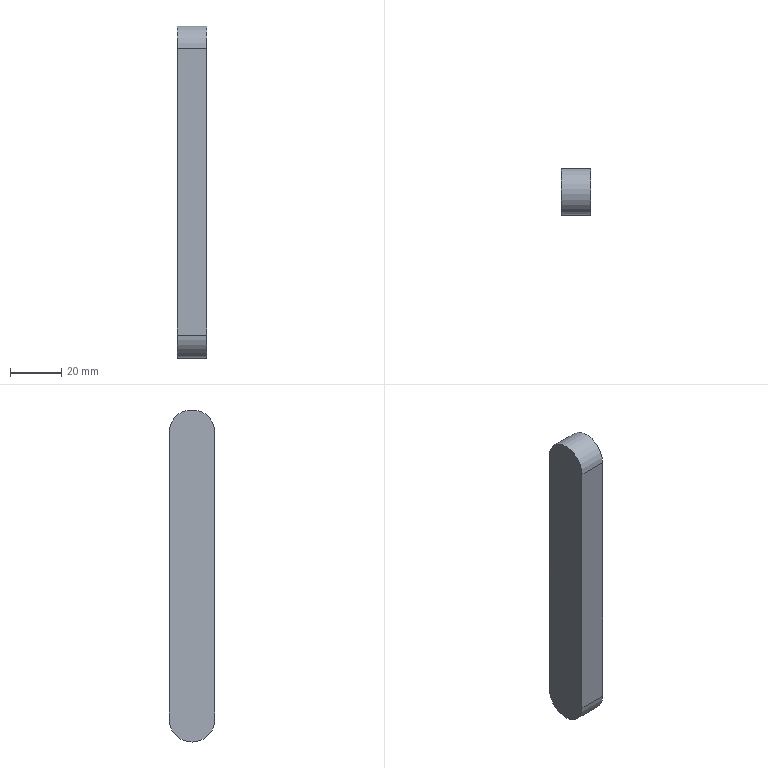Part | SolidWorks | features BaseBody 1 | 1 solid | 7 faces | box 11.4 x 18 x 130 mm | volume 25883 mm3 | plane 4 | cylinder 3 | commonest cylinder face diameters 18 x3
STEP:
#1=CARTESIAN_POINT('',(-168.339,862.249,861.107));
#2=VERTEX_POINT('',#1);
#3=CARTESIAN_POINT('',(-156.939,862.249,861.107));
#4=VERTEX_POINT('',#3);
#5=CARTESIAN_POINT('',(-168.339,862.249,861.107));
#6=DIRECTION('',(1.,0.,0.));
#7=VECTOR('',#6,1000.);
#8=LINE('',#5,#7);
#9=EDGE_CURVE('',#2,#4,#8,.T.);
#10=ORIENTED_EDGE('',*,*,#9,.F.);
#11=CARTESIAN_POINT('',(-168.339,844.249,861.107));
#12=VERTEX_POINT('',#11);
#13=CARTESIAN_POINT('',(-168.339,853.249,861.107));
#14=DIRECTION('',(-1.,0.,0.));
#15=DIRECTION('',(0.,0.,1.));
#16=AXIS2_PLACEMENT_3D('',#13,#14,#15);
#17=CIRCLE('',#16,9.);
#18=EDGE_CURVE('',#12,#2,#17,.T.);
#19=ORIENTED_EDGE('',*,*,#18,.F.);
#20=CARTESIAN_POINT('',(-156.939,844.249,861.107));
#21=VERTEX_POINT('',#20);
#22=CARTESIAN_POINT('',(-168.339,844.249,861.107));
#23=DIRECTION('',(-1.,0.,0.));
#24=VECTOR('',#23,1000.);
#25=LINE('',#22,#24);
#26=EDGE_CURVE('',#21,#12,#25,.T.);
#27=ORIENTED_EDGE('',*,*,#26,.F.);
#28=CARTESIAN_POINT('',(-156.939,853.249,861.107));
#29=DIRECTION('',(1.,0.,0.));
#30=DIRECTION('',(0.,0.,1.));
#31=AXIS2_PLACEMENT_3D('',#28,#29,#30);
#32=CIRCLE('',#31,9.);
#33=EDGE_CURVE('',#4,#21,#32,.T.);
#34=ORIENTED_EDGE('',*,*,#33,.F.);
#35=EDGE_LOOP('',(#10,#19,#27,#34));
#36=FACE_OUTER_BOUND('',#35,.T.);
#37=CARTESIAN_POINT('',(-168.339,853.249,861.107));
#38=DIRECTION('',(1.,0.,0.));
#39=DIRECTION('',(0.,0.,-1.));
#40=AXIS2_PLACEMENT_3D('',#37,#38,#39);
#41=CYLINDRICAL_SURFACE('',#40,9.);
#42=ADVANCED_FACE('',(#36),#41,.T.);
#43=CARTESIAN_POINT('',(-168.339,853.249,740.107));
#44=VERTEX_POINT('',#43);
#45=CARTESIAN_POINT('',(-156.939,853.249,740.107));
#46=VERTEX_POINT('',#45);
#47=CARTESIAN_POINT('',(-168.339,853.249,740.107));
#48=DIRECTION('',(1.,0.,0.));
#49=VECTOR('',#48,1000.);
#50=LINE('',#47,#49);
#51=EDGE_CURVE('',#44,#46,#50,.T.);
#52=ORIENTED_EDGE('',*,*,#51,.F.);
#53=CARTESIAN_POINT('',(-168.339,862.249,749.107));
#54=VERTEX_POINT('',#53);
#55=CARTESIAN_POINT('',(-168.339,853.249,749.107));
#56=DIRECTION('',(-1.,0.,0.));
#57=DIRECTION('',(0.,0.,1.));
#58=AXIS2_PLACEMENT_3D('',#55,#56,#57);
#59=CIRCLE('',#58,9.);
#60=EDGE_CURVE('',#54,#44,#59,.T.);
#61=ORIENTED_EDGE('',*,*,#60,.F.);
#62=CARTESIAN_POINT('',(-156.939,862.249,749.107));
#63=VERTEX_POINT('',#62);
#64=CARTESIAN_POINT('',(-168.339,862.249,749.107));
#65=DIRECTION('',(-1.,0.,0.));
#66=VECTOR('',#65,1000.);
#67=LINE('',#64,#66);
#68=EDGE_CURVE('',#63,#54,#67,.T.);
#69=ORIENTED_EDGE('',*,*,#68,.F.);
#70=CARTESIAN_POINT('',(-156.939,853.249,749.107));
#71=DIRECTION('',(1.,0.,0.));
#72=DIRECTION('',(0.,0.,1.));
#73=AXIS2_PLACEMENT_3D('',#70,#71,#72);
#74=CIRCLE('',#73,9.);
#75=EDGE_CURVE('',#46,#63,#74,.T.);
#76=ORIENTED_EDGE('',*,*,#75,.F.);
#77=EDGE_LOOP('',(#52,#61,#69,#76));
#78=FACE_OUTER_BOUND('',#77,.T.);
#79=CARTESIAN_POINT('',(-168.339,853.249,749.107));
#80=DIRECTION('',(1.,0.,0.));
#81=DIRECTION('',(0.,0.,-1.));
#82=AXIS2_PLACEMENT_3D('',#79,#80,#81);
#83=CYLINDRICAL_SURFACE('',#82,9.);
#84=ADVANCED_FACE('',(#78),#83,.T.);
#85=CARTESIAN_POINT('',(-156.939,844.249,749.107));
#86=VERTEX_POINT('',#85);
#87=CARTESIAN_POINT('',(-156.939,844.249,681.154));
#88=DIRECTION('',(0.,0.,-1.));
#89=VECTOR('',#88,1000.);
#90=LINE('',#87,#89);
#91=EDGE_CURVE('',#21,#86,#90,.T.);
#92=ORIENTED_EDGE('',*,*,#91,.T.);
#93=CARTESIAN_POINT('',(-156.939,853.249,749.107));
#94=DIRECTION('',(1.,0.,0.));
#95=DIRECTION('',(0.,0.,1.));
#96=AXIS2_PLACEMENT_3D('',#93,#94,#95);
#97=CIRCLE('',#96,9.);
#98=EDGE_CURVE('',#86,#46,#97,.T.);
#99=ORIENTED_EDGE('',*,*,#98,.T.);
#100=ORIENTED_EDGE('',*,*,#75,.T.);
#101=CARTESIAN_POINT('',(-156.939,862.249,681.154));
#102=DIRECTION('',(0.,0.,1.));
#103=VECTOR('',#102,1000.);
#104=LINE('',#101,#103);
#105=EDGE_CURVE('',#63,#4,#104,.T.);
#106=ORIENTED_EDGE('',*,*,#105,.T.);
#107=ORIENTED_EDGE('',*,*,#33,.T.);
#108=EDGE_LOOP('',(#92,#99,#100,#106,#107));
#109=FACE_OUTER_BOUND('',#108,.T.);
#110=CARTESIAN_POINT('',(-156.939,845.249,681.154));
#111=DIRECTION('',(-1.,0.,0.));
#112=DIRECTION('',(0.,0.,1.));
#113=AXIS2_PLACEMENT_3D('',#110,#111,#112);
#114=PLANE('',#113);
#115=ADVANCED_FACE('',(#109),#114,.F.);
#116=ORIENTED_EDGE('',*,*,#60,.T.);
#117=CARTESIAN_POINT('',(-168.339,844.249,749.107));
#118=VERTEX_POINT('',#117);
#119=CARTESIAN_POINT('',(-168.339,853.249,749.107));
#120=DIRECTION('',(-1.,0.,0.));
#121=DIRECTION('',(0.,0.,1.));
#122=AXIS2_PLACEMENT_3D('',#119,#120,#121);
#123=CIRCLE('',#122,9.);
#124=EDGE_CURVE('',#44,#118,#123,.T.);
#125=ORIENTED_EDGE('',*,*,#124,.T.);
#126=CARTESIAN_POINT('',(-168.339,844.249,681.154));
#127=DIRECTION('',(0.,0.,-1.));
#128=VECTOR('',#127,1000.);
#129=LINE('',#126,#128);
#130=EDGE_CURVE('',#12,#118,#129,.T.);
#131=ORIENTED_EDGE('',*,*,#130,.F.);
#132=ORIENTED_EDGE('',*,*,#18,.T.);
#133=CARTESIAN_POINT('',(-168.339,862.249,681.154));
#134=DIRECTION('',(0.,0.,1.));
#135=VECTOR('',#134,1000.);
#136=LINE('',#133,#135);
#137=EDGE_CURVE('',#54,#2,#136,.T.);
#138=ORIENTED_EDGE('',*,*,#137,.F.);
#139=EDGE_LOOP('',(#116,#125,#131,#132,#138));
#140=FACE_OUTER_BOUND('',#139,.T.);
#141=CARTESIAN_POINT('',(-168.339,845.249,681.154));
#142=DIRECTION('',(-1.,0.,0.));
#143=DIRECTION('',(0.,0.,1.));
#144=AXIS2_PLACEMENT_3D('',#141,#142,#143);
#145=PLANE('',#144);
#146=ADVANCED_FACE('',(#140),#145,.T.);
#147=ORIENTED_EDGE('',*,*,#130,.T.);
#148=CARTESIAN_POINT('',(-168.339,844.249,749.107));
#149=DIRECTION('',(1.,0.,0.));
#150=VECTOR('',#149,1000.);
#151=LINE('',#148,#150);
#152=EDGE_CURVE('',#118,#86,#151,.T.);
#153=ORIENTED_EDGE('',*,*,#152,.T.);
#154=ORIENTED_EDGE('',*,*,#91,.F.);
#155=ORIENTED_EDGE('',*,*,#26,.T.);
#156=EDGE_LOOP('',(#147,#153,#154,#155));
#157=FACE_OUTER_BOUND('',#156,.T.);
#158=CARTESIAN_POINT('',(-168.339,844.249,681.154));
#159=DIRECTION('',(0.,1.,0.));
#160=DIRECTION('',(1.,0.,0.));
#161=AXIS2_PLACEMENT_3D('',#158,#159,#160);
#162=PLANE('',#161);
#163=ADVANCED_FACE('',(#157),#162,.F.);
#164=ORIENTED_EDGE('',*,*,#105,.F.);
#165=ORIENTED_EDGE('',*,*,#68,.T.);
#166=ORIENTED_EDGE('',*,*,#137,.T.);
#167=ORIENTED_EDGE('',*,*,#9,.T.);
#168=EDGE_LOOP('',(#164,#165,#166,#167));
#169=FACE_OUTER_BOUND('',#168,.T.);
#170=CARTESIAN_POINT('',(-168.339,862.249,681.154));
#171=DIRECTION('',(0.,-1.,0.));
#172=DIRECTION('',(0.,0.,-1.));
#173=AXIS2_PLACEMENT_3D('',#170,#171,#172);
#174=PLANE('',#173);
#175=ADVANCED_FACE('',(#169),#174,.F.);
#176=ORIENTED_EDGE('',*,*,#124,.F.);
#177=ORIENTED_EDGE('',*,*,#51,.T.);
#178=ORIENTED_EDGE('',*,*,#98,.F.);
#179=ORIENTED_EDGE('',*,*,#152,.F.);
#180=EDGE_LOOP('',(#176,#177,#178,#179));
#181=FACE_OUTER_BOUND('',#180,.T.);
#182=CARTESIAN_POINT('',(-168.339,853.249,749.107));
#183=DIRECTION('',(1.,0.,0.));
#184=DIRECTION('',(0.,0.,-1.));
#185=AXIS2_PLACEMENT_3D('',#182,#183,#184);
#186=CYLINDRICAL_SURFACE('',#185,9.);
#187=ADVANCED_FACE('',(#181),#186,.T.);
#188=CLOSED_SHELL('',(#42,#84,#115,#146,#163,#175,#187));
#189=MANIFOLD_SOLID_BREP('',#188);
#190=CARTESIAN_POINT('',(0.,0.,0.));
#191=DIRECTION('',(0.,0.,1.));
#192=DIRECTION('',(1.,0.,0.));
#193=AXIS2_PLACEMENT_3D('',#190,#191,#192);
#194=(LENGTH_UNIT()NAMED_UNIT(*)SI_UNIT(.MILLI.,.METRE.));
#195=UNCERTAINTY_MEASURE_WITH_UNIT(LENGTH_MEASURE(0.00001),#194,'','');
#196=(NAMED_UNIT(*)PLANE_ANGLE_UNIT()SI_UNIT($,.RADIAN.));
#197=(NAMED_UNIT(*)SI_UNIT($,.STERADIAN.)SOLID_ANGLE_UNIT());
#198=(GEOMETRIC_REPRESENTATION_CONTEXT(3)GLOBAL_UNCERTAINTY_ASSIGNED_CONTEXT((#195))GLOBAL_UNIT_ASSIGNED_CONTEXT((#194,#196,#197))REPRESENTATION_CONTEXT('',''));
#199=ADVANCED_BREP_SHAPE_REPRESENTATION('',(#189,#193),#198);